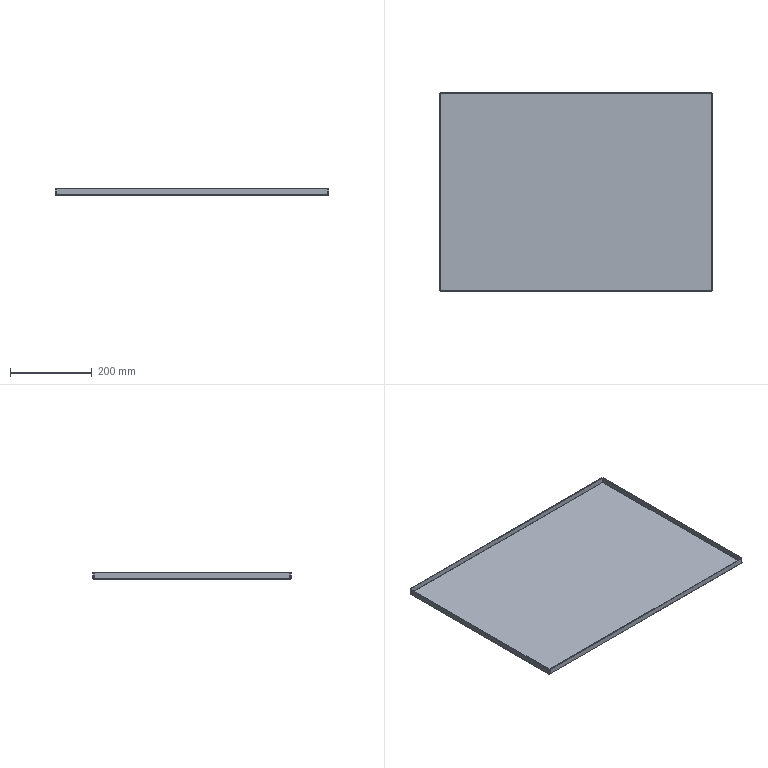Part | SolidWorks | 1 solid | 38 faces | box 670 x 485 x 15 mm | volume 707189 mm3 | plane 22 | spline 8 | cylinder 8 | commonest cylinder face diameters 0.2 x4 4.2 x4
STEP:
#1=CARTESIAN_POINT('',(332.9,-240.4,-2.));
#2=VERTEX_POINT('',#1);
#3=CARTESIAN_POINT('',(-332.9,-240.4,-2.));
#4=VERTEX_POINT('',#3);
#5=CARTESIAN_POINT('',(332.9,-240.4,-2.));
#6=DIRECTION('',(-1.,0.,0.));
#7=VECTOR('',#6,1000.);
#8=LINE('',#5,#7);
#9=EDGE_CURVE('',#2,#4,#8,.T.);
#10=ORIENTED_EDGE('',*,*,#9,.T.);
#11=CARTESIAN_POINT('',(-332.9,240.4,-2.));
#12=VERTEX_POINT('',#11);
#13=CARTESIAN_POINT('',(-332.9,-240.4,-2.));
#14=DIRECTION('',(0.,1.,0.));
#15=VECTOR('',#14,1000.);
#16=LINE('',#13,#15);
#17=EDGE_CURVE('',#4,#12,#16,.T.);
#18=ORIENTED_EDGE('',*,*,#17,.T.);
#19=CARTESIAN_POINT('',(332.9,240.4,-2.));
#20=VERTEX_POINT('',#19);
#21=CARTESIAN_POINT('',(-332.9,240.4,-2.));
#22=DIRECTION('',(1.,0.,0.));
#23=VECTOR('',#22,1000.);
#24=LINE('',#21,#23);
#25=EDGE_CURVE('',#12,#20,#24,.T.);
#26=ORIENTED_EDGE('',*,*,#25,.T.);
#27=CARTESIAN_POINT('',(332.9,240.4,-2.));
#28=DIRECTION('',(0.,-1.,0.));
#29=VECTOR('',#28,1000.);
#30=LINE('',#27,#29);
#31=EDGE_CURVE('',#20,#2,#30,.T.);
#32=ORIENTED_EDGE('',*,*,#31,.T.);
#33=EDGE_LOOP('',(#10,#18,#26,#32));
#34=FACE_OUTER_BOUND('',#33,.T.);
#35=CARTESIAN_POINT('',(0.,0.,-2.));
#36=DIRECTION('',(0.,0.,1.));
#37=DIRECTION('',(1.,0.,0.));
#38=AXIS2_PLACEMENT_3D('',#35,#36,#37);
#39=PLANE('',#38);
#40=ADVANCED_FACE('',(#34),#39,.F.);
#41=CARTESIAN_POINT('',(-332.9,-240.4,0.));
#42=VERTEX_POINT('',#41);
#43=CARTESIAN_POINT('',(-332.9,240.4,0.));
#44=VERTEX_POINT('',#43);
#45=CARTESIAN_POINT('',(-332.9,-240.4,0.));
#46=DIRECTION('',(0.,1.,0.));
#47=VECTOR('',#46,1000.);
#48=LINE('',#45,#47);
#49=EDGE_CURVE('',#42,#44,#48,.T.);
#50=ORIENTED_EDGE('',*,*,#49,.F.);
#51=CARTESIAN_POINT('',(332.9,-240.4,0.));
#52=VERTEX_POINT('',#51);
#53=CARTESIAN_POINT('',(332.9,-240.4,0.));
#54=DIRECTION('',(-1.,0.,0.));
#55=VECTOR('',#54,1000.);
#56=LINE('',#53,#55);
#57=EDGE_CURVE('',#52,#42,#56,.T.);
#58=ORIENTED_EDGE('',*,*,#57,.F.);
#59=CARTESIAN_POINT('',(332.9,240.4,0.));
#60=VERTEX_POINT('',#59);
#61=CARTESIAN_POINT('',(332.9,240.4,0.));
#62=DIRECTION('',(0.,-1.,0.));
#63=VECTOR('',#62,1000.);
#64=LINE('',#61,#63);
#65=EDGE_CURVE('',#60,#52,#64,.T.);
#66=ORIENTED_EDGE('',*,*,#65,.F.);
#67=CARTESIAN_POINT('',(-332.9,240.4,0.));
#68=DIRECTION('',(1.,0.,0.));
#69=VECTOR('',#68,1000.);
#70=LINE('',#67,#69);
#71=EDGE_CURVE('',#44,#60,#70,.T.);
#72=ORIENTED_EDGE('',*,*,#71,.F.);
#73=EDGE_LOOP('',(#50,#58,#66,#72));
#74=FACE_OUTER_BOUND('',#73,.T.);
#75=CARTESIAN_POINT('',(0.,0.,0.));
#76=DIRECTION('',(0.,0.,1.));
#77=DIRECTION('',(1.,0.,0.));
#78=AXIS2_PLACEMENT_3D('',#75,#76,#77);
#79=PLANE('',#78);
#80=ADVANCED_FACE('',(#74),#79,.T.);
#81=CARTESIAN_POINT('',(-335.,239.793,0.1));
#82=VERTEX_POINT('',#81);
#83=CARTESIAN_POINT('',(-333.,239.793,0.1));
#84=VERTEX_POINT('',#83);
#85=CARTESIAN_POINT('',(-333.,239.793,0.1));
#86=DIRECTION('',(1.,0.,0.));
#87=VECTOR('',#86,1000.);
#88=LINE('',#85,#87);
#89=EDGE_CURVE('',#82,#84,#88,.T.);
#90=ORIENTED_EDGE('',*,*,#89,.T.);
#91=CARTESIAN_POINT('',(-332.9,240.4,0.));
#92=CARTESIAN_POINT('',(-332.926,240.299,0.));
#93=CARTESIAN_POINT('',(-332.952,240.198,0.01078));
#94=CARTESIAN_POINT('',(-332.989,239.995,0.0478));
#95=CARTESIAN_POINT('',(-333.,239.894,0.07382));
#96=CARTESIAN_POINT('',(-333.,239.793,0.1));
#97=B_SPLINE_CURVE_WITH_KNOTS('',3,(#91,#92,#93,#94,#95,#96),.UNSPECIFIED.,.F.,.F.,(4,2,4),(0.,0.5,1.),.UNSPECIFIED.);
#98=EDGE_CURVE('',#44,#84,#97,.T.);
#99=ORIENTED_EDGE('',*,*,#98,.F.);
#100=CARTESIAN_POINT('',(-332.9,240.4,0.));
#101=DIRECTION('',(0.,0.,-1.));
#102=VECTOR('',#101,1000.);
#103=LINE('',#100,#102);
#104=EDGE_CURVE('',#44,#12,#103,.T.);
#105=ORIENTED_EDGE('',*,*,#104,.T.);
#106=CARTESIAN_POINT('',(-332.9,240.4,-2.));
#107=CARTESIAN_POINT('',(-333.039,240.374,-2.));
#108=CARTESIAN_POINT('',(-333.175,240.349,-1.986));
#109=CARTESIAN_POINT('',(-333.443,240.299,-1.933));
#110=CARTESIAN_POINT('',(-333.576,240.274,-1.893));
#111=CARTESIAN_POINT('',(-333.831,240.223,-1.787));
#112=CARTESIAN_POINT('',(-333.951,240.198,-1.723));
#113=CARTESIAN_POINT('',(-334.179,240.147,-1.571));
#114=CARTESIAN_POINT('',(-334.287,240.122,-1.482));
#115=CARTESIAN_POINT('',(-334.481,240.071,-1.289));
#116=CARTESIAN_POINT('',(-334.568,240.046,-1.183));
#117=CARTESIAN_POINT('',(-334.721,239.996,-0.9542));
#118=CARTESIAN_POINT('',(-334.787,239.97,-0.8315));
#119=CARTESIAN_POINT('',(-334.944,239.895,-0.4527));
#120=CARTESIAN_POINT('',(-335.,239.844,-0.1773));
#121=CARTESIAN_POINT('',(-335.,239.793,0.1));
#122=B_SPLINE_CURVE_WITH_KNOTS('',3,(#106,#107,#108,#109,#110,#111,#112,#113,#114,#115,#116,#117,#118,#119,#120,#121),.UNSPECIFIED.,.F.,.F.,(4,2,2,2,2,2,2,4),(0.,0.0004169,0.0008339,0.001251,0.001668,0.002085,0.002502,0.003336),.UNSPECIFIED.);
#123=EDGE_CURVE('',#12,#82,#122,.T.);
#124=ORIENTED_EDGE('',*,*,#123,.T.);
#125=EDGE_LOOP('',(#90,#99,#105,#124));
#126=FACE_OUTER_BOUND('',#125,.T.);
#127=CARTESIAN_POINT('',(-332.9,240.4,-2.02));
#128=CARTESIAN_POINT('',(-333.178,240.349,-2.02));
#129=CARTESIAN_POINT('',(-333.455,240.299,-1.965));
#130=CARTESIAN_POINT('',(-333.968,240.198,-1.752));
#131=CARTESIAN_POINT('',(-334.203,240.147,-1.595));
#132=CARTESIAN_POINT('',(-334.595,240.046,-1.203));
#133=CARTESIAN_POINT('',(-334.752,239.995,-0.9677));
#134=CARTESIAN_POINT('',(-334.965,239.894,-0.4549));
#135=CARTESIAN_POINT('',(-335.02,239.843,-0.1776));
#136=CARTESIAN_POINT('',(-335.02,239.793,0.1));
#137=CARTESIAN_POINT('',(-332.9,240.4,-2.));
#138=CARTESIAN_POINT('',(-333.175,240.349,-2.));
#139=CARTESIAN_POINT('',(-333.45,240.299,-1.945));
#140=CARTESIAN_POINT('',(-333.958,240.198,-1.735));
#141=CARTESIAN_POINT('',(-334.191,240.147,-1.579));
#142=CARTESIAN_POINT('',(-334.579,240.046,-1.191));
#143=CARTESIAN_POINT('',(-334.735,239.995,-0.9576));
#144=CARTESIAN_POINT('',(-334.945,239.894,-0.4497));
#145=CARTESIAN_POINT('',(-335.,239.843,-0.1749));
#146=CARTESIAN_POINT('',(-335.,239.793,0.1));
#147=CARTESIAN_POINT('',(-332.9,240.4,0.));
#148=CARTESIAN_POINT('',(-332.913,240.349,0.));
#149=CARTESIAN_POINT('',(-332.926,240.299,0.002603));
#150=CARTESIAN_POINT('',(-332.95,240.198,0.01262));
#151=CARTESIAN_POINT('',(-332.961,240.147,0.02003));
#152=CARTESIAN_POINT('',(-332.98,240.046,0.03855));
#153=CARTESIAN_POINT('',(-332.987,239.995,0.04964));
#154=CARTESIAN_POINT('',(-332.997,239.894,0.07383));
#155=CARTESIAN_POINT('',(-333.,239.843,0.08691));
#156=CARTESIAN_POINT('',(-333.,239.793,0.1));
#157=B_SPLINE_SURFACE_WITH_KNOTS('',1,3,((#127,#128,#129,#130,#131,#132,#133,#134,#135,#136),(#137,#138,#139,#140,#141,#142,#143,#144,#145,#146),(#147,#148,#149,#150,#151,#152,#153,#154,#155,#156)),.UNSPECIFIED.,.F.,.F.,.F.,(2,1,2),(4,2,2,2,4),(-0.01,0.,1.),(0.,0.25,0.5,0.75,1.),.UNSPECIFIED.);
#158=ADVANCED_FACE('',(#126),#157,.F.);
#159=CARTESIAN_POINT('',(-333.,-239.793,0.1));
#160=VERTEX_POINT('',#159);
#161=CARTESIAN_POINT('',(-333.,-239.793,0.1));
#162=CARTESIAN_POINT('',(-333.,-239.894,0.07382));
#163=CARTESIAN_POINT('',(-332.989,-239.995,0.0478));
#164=CARTESIAN_POINT('',(-332.952,-240.198,0.01078));
#165=CARTESIAN_POINT('',(-332.926,-240.299,0.));
#166=CARTESIAN_POINT('',(-332.9,-240.4,0.));
#167=B_SPLINE_CURVE_WITH_KNOTS('',3,(#161,#162,#163,#164,#165,#166),.UNSPECIFIED.,.F.,.F.,(4,2,4),(0.,0.5,1.),.UNSPECIFIED.);
#168=EDGE_CURVE('',#160,#42,#167,.T.);
#169=ORIENTED_EDGE('',*,*,#168,.F.);
#170=CARTESIAN_POINT('',(-335.,-239.793,0.1));
#171=VERTEX_POINT('',#170);
#172=CARTESIAN_POINT('',(-333.,-239.793,0.1));
#173=DIRECTION('',(1.,0.,0.));
#174=VECTOR('',#173,1000.);
#175=LINE('',#172,#174);
#176=EDGE_CURVE('',#171,#160,#175,.T.);
#177=ORIENTED_EDGE('',*,*,#176,.F.);
#178=CARTESIAN_POINT('',(-335.,-239.793,0.1));
#179=CARTESIAN_POINT('',(-335.,-239.818,-0.03865));
#180=CARTESIAN_POINT('',(-334.986,-239.844,-0.175));
#181=CARTESIAN_POINT('',(-334.933,-239.894,-0.4432));
#182=CARTESIAN_POINT('',(-334.893,-239.919,-0.5764));
#183=CARTESIAN_POINT('',(-334.787,-239.97,-0.8308));
#184=CARTESIAN_POINT('',(-334.723,-239.995,-0.9514));
#185=CARTESIAN_POINT('',(-334.571,-240.045,-1.179));
#186=CARTESIAN_POINT('',(-334.482,-240.071,-1.287));
#187=CARTESIAN_POINT('',(-334.289,-240.122,-1.481));
#188=CARTESIAN_POINT('',(-334.183,-240.147,-1.568));
#189=CARTESIAN_POINT('',(-333.954,-240.197,-1.721));
#190=CARTESIAN_POINT('',(-333.832,-240.223,-1.787));
#191=CARTESIAN_POINT('',(-333.453,-240.298,-1.944));
#192=CARTESIAN_POINT('',(-333.177,-240.349,-2.));
#193=CARTESIAN_POINT('',(-332.9,-240.4,-2.));
#194=B_SPLINE_CURVE_WITH_KNOTS('',3,(#178,#179,#180,#181,#182,#183,#184,#185,#186,#187,#188,#189,#190,#191,#192,#193),.UNSPECIFIED.,.F.,.F.,(4,2,2,2,2,2,2,4),(0.,0.0004169,0.0008339,0.001251,0.001668,0.002085,0.002502,0.003336),.UNSPECIFIED.);
#195=EDGE_CURVE('',#171,#4,#194,.T.);
#196=ORIENTED_EDGE('',*,*,#195,.T.);
#197=CARTESIAN_POINT('',(-332.9,-240.4,0.));
#198=DIRECTION('',(0.,0.,-1.));
#199=VECTOR('',#198,1000.);
#200=LINE('',#197,#199);
#201=EDGE_CURVE('',#42,#4,#200,.T.);
#202=ORIENTED_EDGE('',*,*,#201,.F.);
#203=EDGE_LOOP('',(#169,#177,#196,#202));
#204=FACE_OUTER_BOUND('',#203,.T.);
#205=CARTESIAN_POINT('',(-335.02,-239.793,0.1));
#206=CARTESIAN_POINT('',(-335.02,-239.843,-0.1776));
#207=CARTESIAN_POINT('',(-334.965,-239.894,-0.4549));
#208=CARTESIAN_POINT('',(-334.752,-239.995,-0.9677));
#209=CARTESIAN_POINT('',(-334.595,-240.046,-1.203));
#210=CARTESIAN_POINT('',(-334.203,-240.147,-1.595));
#211=CARTESIAN_POINT('',(-333.968,-240.198,-1.752));
#212=CARTESIAN_POINT('',(-333.455,-240.299,-1.965));
#213=CARTESIAN_POINT('',(-333.178,-240.349,-2.02));
#214=CARTESIAN_POINT('',(-332.9,-240.4,-2.02));
#215=CARTESIAN_POINT('',(-335.,-239.793,0.1));
#216=CARTESIAN_POINT('',(-335.,-239.843,-0.1749));
#217=CARTESIAN_POINT('',(-334.945,-239.894,-0.4497));
#218=CARTESIAN_POINT('',(-334.735,-239.995,-0.9576));
#219=CARTESIAN_POINT('',(-334.579,-240.046,-1.191));
#220=CARTESIAN_POINT('',(-334.191,-240.147,-1.579));
#221=CARTESIAN_POINT('',(-333.958,-240.198,-1.735));
#222=CARTESIAN_POINT('',(-333.45,-240.299,-1.945));
#223=CARTESIAN_POINT('',(-333.175,-240.349,-2.));
#224=CARTESIAN_POINT('',(-332.9,-240.4,-2.));
#225=CARTESIAN_POINT('',(-333.,-239.793,0.1));
#226=CARTESIAN_POINT('',(-333.,-239.843,0.08691));
#227=CARTESIAN_POINT('',(-332.997,-239.894,0.07383));
#228=CARTESIAN_POINT('',(-332.987,-239.995,0.04964));
#229=CARTESIAN_POINT('',(-332.98,-240.046,0.03855));
#230=CARTESIAN_POINT('',(-332.961,-240.147,0.02003));
#231=CARTESIAN_POINT('',(-332.95,-240.198,0.01262));
#232=CARTESIAN_POINT('',(-332.926,-240.299,0.002603));
#233=CARTESIAN_POINT('',(-332.913,-240.349,0.));
#234=CARTESIAN_POINT('',(-332.9,-240.4,0.));
#235=B_SPLINE_SURFACE_WITH_KNOTS('',1,3,((#205,#206,#207,#208,#209,#210,#211,#212,#213,#214),(#215,#216,#217,#218,#219,#220,#221,#222,#223,#224),(#225,#226,#227,#228,#229,#230,#231,#232,#233,#234)),.UNSPECIFIED.,.F.,.F.,.F.,(2,1,2),(4,2,2,2,4),(-0.01,0.,1.),(0.,0.25,0.5,0.75,1.),.UNSPECIFIED.);
#236=ADVANCED_FACE('',(#204),#235,.F.);
#237=ORIENTED_EDGE('',*,*,#17,.F.);
#238=ORIENTED_EDGE('',*,*,#195,.F.);
#239=CARTESIAN_POINT('',(-335.,242.5,0.1));
#240=DIRECTION('',(0.,1.,0.));
#241=VECTOR('',#240,1000.);
#242=LINE('',#239,#241);
#243=EDGE_CURVE('',#171,#82,#242,.T.);
#244=ORIENTED_EDGE('',*,*,#243,.T.);
#245=ORIENTED_EDGE('',*,*,#123,.F.);
#246=EDGE_LOOP('',(#237,#238,#244,#245));
#247=FACE_OUTER_BOUND('',#246,.T.);
#248=CARTESIAN_POINT('',(-332.9,-240.4,0.1));
#249=DIRECTION('',(0.,-1.,0.));
#250=DIRECTION('',(-1.,0.,0.));
#251=AXIS2_PLACEMENT_3D('',#248,#249,#250);
#252=CYLINDRICAL_SURFACE('',#251,2.1);
#253=ADVANCED_FACE('',(#247),#252,.T.);
#254=ORIENTED_EDGE('',*,*,#49,.T.);
#255=ORIENTED_EDGE('',*,*,#98,.T.);
#256=CARTESIAN_POINT('',(-333.,242.5,0.1));
#257=DIRECTION('',(0.,-1.,0.));
#258=VECTOR('',#257,1000.);
#259=LINE('',#256,#258);
#260=EDGE_CURVE('',#84,#160,#259,.T.);
#261=ORIENTED_EDGE('',*,*,#260,.T.);
#262=ORIENTED_EDGE('',*,*,#168,.T.);
#263=EDGE_LOOP('',(#254,#255,#261,#262));
#264=FACE_OUTER_BOUND('',#263,.T.);
#265=CARTESIAN_POINT('',(-332.9,-240.4,0.1));
#266=DIRECTION('',(0.,-1.,0.));
#267=DIRECTION('',(-1.,0.,0.));
#268=AXIS2_PLACEMENT_3D('',#265,#266,#267);
#269=CYLINDRICAL_SURFACE('',#268,0.1);
#270=ADVANCED_FACE('',(#264),#269,.F.);
#271=CARTESIAN_POINT('',(-335.,239.793,13.));
#272=VERTEX_POINT('',#271);
#273=CARTESIAN_POINT('',(-335.,239.793,0.));
#274=DIRECTION('',(0.,0.,1.));
#275=VECTOR('',#274,1000.);
#276=LINE('',#273,#275);
#277=EDGE_CURVE('',#82,#272,#276,.T.);
#278=ORIENTED_EDGE('',*,*,#277,.T.);
#279=CARTESIAN_POINT('',(-333.,239.793,13.));
#280=VERTEX_POINT('',#279);
#281=CARTESIAN_POINT('',(-333.,239.793,13.));
#282=DIRECTION('',(1.,0.,0.));
#283=VECTOR('',#282,1000.);
#284=LINE('',#281,#283);
#285=EDGE_CURVE('',#272,#280,#284,.T.);
#286=ORIENTED_EDGE('',*,*,#285,.T.);
#287=CARTESIAN_POINT('',(-333.,239.793,0.));
#288=DIRECTION('',(0.,0.,1.));
#289=VECTOR('',#288,1000.);
#290=LINE('',#287,#289);
#291=EDGE_CURVE('',#84,#280,#290,.T.);
#292=ORIENTED_EDGE('',*,*,#291,.F.);
#293=ORIENTED_EDGE('',*,*,#89,.F.);
#294=EDGE_LOOP('',(#278,#286,#292,#293));
#295=FACE_OUTER_BOUND('',#294,.T.);
#296=CARTESIAN_POINT('',(-333.,239.793,0.));
#297=DIRECTION('',(0.,1.,0.));
#298=DIRECTION('',(0.,0.,1.));
#299=AXIS2_PLACEMENT_3D('',#296,#297,#298);
#300=PLANE('',#299);
#301=ADVANCED_FACE('',(#295),#300,.T.);
#302=ORIENTED_EDGE('',*,*,#243,.F.);
#303=CARTESIAN_POINT('',(-335.,-239.793,13.));
#304=VERTEX_POINT('',#303);
#305=CARTESIAN_POINT('',(-335.,-239.793,0.));
#306=DIRECTION('',(0.,0.,1.));
#307=VECTOR('',#306,1000.);
#308=LINE('',#305,#307);
#309=EDGE_CURVE('',#171,#304,#308,.T.);
#310=ORIENTED_EDGE('',*,*,#309,.T.);
#311=CARTESIAN_POINT('',(-335.,0.,13.));
#312=DIRECTION('',(0.,1.,0.));
#313=VECTOR('',#312,1000.);
#314=LINE('',#311,#313);
#315=EDGE_CURVE('',#304,#272,#314,.T.);
#316=ORIENTED_EDGE('',*,*,#315,.T.);
#317=ORIENTED_EDGE('',*,*,#277,.F.);
#318=EDGE_LOOP('',(#302,#310,#316,#317));
#319=FACE_OUTER_BOUND('',#318,.T.);
#320=CARTESIAN_POINT('',(-335.,0.,0.));
#321=DIRECTION('',(1.,0.,0.));
#322=DIRECTION('',(0.,0.,-1.));
#323=AXIS2_PLACEMENT_3D('',#320,#321,#322);
#324=PLANE('',#323);
#325=ADVANCED_FACE('',(#319),#324,.F.);
#326=CARTESIAN_POINT('',(-333.,-239.793,13.));
#327=VERTEX_POINT('',#326);
#328=CARTESIAN_POINT('',(-333.,-239.793,0.));
#329=DIRECTION('',(0.,0.,1.));
#330=VECTOR('',#329,1000.);
#331=LINE('',#328,#330);
#332=EDGE_CURVE('',#160,#327,#331,.T.);
#333=ORIENTED_EDGE('',*,*,#332,.F.);
#334=ORIENTED_EDGE('',*,*,#260,.F.);
#335=ORIENTED_EDGE('',*,*,#291,.T.);
#336=CARTESIAN_POINT('',(-333.,242.5,13.));
#337=DIRECTION('',(0.,1.,0.));
#338=VECTOR('',#337,1000.);
#339=LINE('',#336,#338);
#340=EDGE_CURVE('',#327,#280,#339,.T.);
#341=ORIENTED_EDGE('',*,*,#340,.F.);
#342=EDGE_LOOP('',(#333,#334,#335,#341));
#343=FACE_OUTER_BOUND('',#342,.T.);
#344=CARTESIAN_POINT('',(-333.,0.,0.));
#345=DIRECTION('',(1.,0.,0.));
#346=DIRECTION('',(0.,0.,-1.));
#347=AXIS2_PLACEMENT_3D('',#344,#345,#346);
#348=PLANE('',#347);
#349=ADVANCED_FACE('',(#343),#348,.T.);
#350=ORIENTED_EDGE('',*,*,#315,.F.);
#351=CARTESIAN_POINT('',(-335.,-239.793,13.));
#352=DIRECTION('',(1.,0.,0.));
#353=VECTOR('',#352,1000.);
#354=LINE('',#351,#353);
#355=EDGE_CURVE('',#304,#327,#354,.T.);
#356=ORIENTED_EDGE('',*,*,#355,.T.);
#357=ORIENTED_EDGE('',*,*,#340,.T.);
#358=ORIENTED_EDGE('',*,*,#285,.F.);
#359=EDGE_LOOP('',(#350,#356,#357,#358));
#360=FACE_OUTER_BOUND('',#359,.T.);
#361=CARTESIAN_POINT('',(-335.,242.5,13.));
#362=DIRECTION('',(0.,0.,-1.));
#363=DIRECTION('',(-1.,0.,0.));
#364=AXIS2_PLACEMENT_3D('',#361,#362,#363);
#365=PLANE('',#364);
#366=ADVANCED_FACE('',(#360),#365,.F.);
#367=ORIENTED_EDGE('',*,*,#355,.F.);
#368=ORIENTED_EDGE('',*,*,#309,.F.);
#369=ORIENTED_EDGE('',*,*,#176,.T.);
#370=ORIENTED_EDGE('',*,*,#332,.T.);
#371=EDGE_LOOP('',(#367,#368,#369,#370));
#372=FACE_OUTER_BOUND('',#371,.T.);
#373=CARTESIAN_POINT('',(-333.,-239.793,0.));
#374=DIRECTION('',(0.,1.,0.));
#375=DIRECTION('',(0.,0.,1.));
#376=AXIS2_PLACEMENT_3D('',#373,#374,#375);
#377=PLANE('',#376);
#378=ADVANCED_FACE('',(#372),#377,.F.);
#379=CARTESIAN_POINT('',(332.293,242.5,0.1));
#380=VERTEX_POINT('',#379);
#381=CARTESIAN_POINT('',(332.293,240.5,0.1));
#382=VERTEX_POINT('',#381);
#383=CARTESIAN_POINT('',(332.293,240.5,0.1));
#384=DIRECTION('',(0.,-1.,0.));
#385=VECTOR('',#384,1000.);
#386=LINE('',#383,#385);
#387=EDGE_CURVE('',#380,#382,#386,.T.);
#388=ORIENTED_EDGE('',*,*,#387,.T.);
#389=CARTESIAN_POINT('',(332.9,240.4,0.));
#390=CARTESIAN_POINT('',(332.799,240.426,0.));
#391=CARTESIAN_POINT('',(332.698,240.452,0.01078));
#392=CARTESIAN_POINT('',(332.495,240.489,0.0478));
#393=CARTESIAN_POINT('',(332.394,240.5,0.07382));
#394=CARTESIAN_POINT('',(332.293,240.5,0.1));
#395=B_SPLINE_CURVE_WITH_KNOTS('',3,(#389,#390,#391,#392,#393,#394),.UNSPECIFIED.,.F.,.F.,(4,2,4),(0.,0.5,1.),.UNSPECIFIED.);
#396=EDGE_CURVE('',#60,#382,#395,.T.);
#397=ORIENTED_EDGE('',*,*,#396,.F.);
#398=CARTESIAN_POINT('',(332.9,240.4,0.));
#399=DIRECTION('',(0.,0.,-1.));
#400=VECTOR('',#399,1000.);
#401=LINE('',#398,#400);
#402=EDGE_CURVE('',#60,#20,#401,.T.);
#403=ORIENTED_EDGE('',*,*,#402,.T.);
#404=CARTESIAN_POINT('',(332.9,240.4,-2.));
#405=CARTESIAN_POINT('',(332.874,240.539,-2.));
#406=CARTESIAN_POINT('',(332.849,240.675,-1.986));
#407=CARTESIAN_POINT('',(332.799,240.943,-1.933));
#408=CARTESIAN_POINT('',(332.774,241.076,-1.893));
#409=CARTESIAN_POINT('',(332.723,241.331,-1.787));
#410=CARTESIAN_POINT('',(332.698,241.451,-1.723));
#411=CARTESIAN_POINT('',(332.647,241.679,-1.571));
#412=CARTESIAN_POINT('',(332.622,241.787,-1.482));
#413=CARTESIAN_POINT('',(332.571,241.981,-1.289));
#414=CARTESIAN_POINT('',(332.546,242.068,-1.183));
#415=CARTESIAN_POINT('',(332.496,242.221,-0.9542));
#416=CARTESIAN_POINT('',(332.47,242.287,-0.8315));
#417=CARTESIAN_POINT('',(332.395,242.444,-0.4527));
#418=CARTESIAN_POINT('',(332.344,242.5,-0.1773));
#419=CARTESIAN_POINT('',(332.293,242.5,0.1));
#420=B_SPLINE_CURVE_WITH_KNOTS('',3,(#404,#405,#406,#407,#408,#409,#410,#411,#412,#413,#414,#415,#416,#417,#418,#419),.UNSPECIFIED.,.F.,.F.,(4,2,2,2,2,2,2,4),(0.,0.0004169,0.0008339,0.001251,0.001668,0.002085,0.002502,0.003336),.UNSPECIFIED.);
#421=EDGE_CURVE('',#20,#380,#420,.T.);
#422=ORIENTED_EDGE('',*,*,#421,.T.);
#423=EDGE_LOOP('',(#388,#397,#403,#422));
#424=FACE_OUTER_BOUND('',#423,.T.);
#425=CARTESIAN_POINT('',(332.9,240.4,-2.02));
#426=CARTESIAN_POINT('',(332.849,240.678,-2.02));
#427=CARTESIAN_POINT('',(332.799,240.955,-1.965));
#428=CARTESIAN_POINT('',(332.698,241.468,-1.752));
#429=CARTESIAN_POINT('',(332.647,241.703,-1.595));
#430=CARTESIAN_POINT('',(332.546,242.095,-1.203));
#431=CARTESIAN_POINT('',(332.495,242.252,-0.9677));
#432=CARTESIAN_POINT('',(332.394,242.465,-0.4549));
#433=CARTESIAN_POINT('',(332.343,242.52,-0.1776));
#434=CARTESIAN_POINT('',(332.293,242.52,0.1));
#435=CARTESIAN_POINT('',(332.9,240.4,-2.));
#436=CARTESIAN_POINT('',(332.849,240.675,-2.));
#437=CARTESIAN_POINT('',(332.799,240.95,-1.945));
#438=CARTESIAN_POINT('',(332.698,241.458,-1.735));
#439=CARTESIAN_POINT('',(332.647,241.691,-1.579));
#440=CARTESIAN_POINT('',(332.546,242.079,-1.191));
#441=CARTESIAN_POINT('',(332.495,242.235,-0.9576));
#442=CARTESIAN_POINT('',(332.394,242.445,-0.4497));
#443=CARTESIAN_POINT('',(332.343,242.5,-0.1749));
#444=CARTESIAN_POINT('',(332.293,242.5,0.1));
#445=CARTESIAN_POINT('',(332.9,240.4,0.));
#446=CARTESIAN_POINT('',(332.849,240.413,0.));
#447=CARTESIAN_POINT('',(332.799,240.426,0.002603));
#448=CARTESIAN_POINT('',(332.698,240.45,0.01262));
#449=CARTESIAN_POINT('',(332.647,240.461,0.02003));
#450=CARTESIAN_POINT('',(332.546,240.48,0.03855));
#451=CARTESIAN_POINT('',(332.495,240.487,0.04964));
#452=CARTESIAN_POINT('',(332.394,240.497,0.07383));
#453=CARTESIAN_POINT('',(332.343,240.5,0.08691));
#454=CARTESIAN_POINT('',(332.293,240.5,0.1));
#455=B_SPLINE_SURFACE_WITH_KNOTS('',1,3,((#425,#426,#427,#428,#429,#430,#431,#432,#433,#434),(#435,#436,#437,#438,#439,#440,#441,#442,#443,#444),(#445,#446,#447,#448,#449,#450,#451,#452,#453,#454)),.UNSPECIFIED.,.F.,.F.,.F.,(2,1,2),(4,2,2,2,4),(-0.01,0.,1.),(0.,0.25,0.5,0.75,1.),.UNSPECIFIED.);
#456=ADVANCED_FACE('',(#424),#455,.F.);
#457=CARTESIAN_POINT('',(-332.293,240.5,0.1));
#458=VERTEX_POINT('',#457);
#459=CARTESIAN_POINT('',(-332.293,240.5,0.1));
#460=CARTESIAN_POINT('',(-332.394,240.5,0.07382));
#461=CARTESIAN_POINT('',(-332.495,240.489,0.0478));
#462=CARTESIAN_POINT('',(-332.698,240.452,0.01078));
#463=CARTESIAN_POINT('',(-332.799,240.426,0.));
#464=CARTESIAN_POINT('',(-332.9,240.4,0.));
#465=B_SPLINE_CURVE_WITH_KNOTS('',3,(#459,#460,#461,#462,#463,#464),.UNSPECIFIED.,.F.,.F.,(4,2,4),(0.,0.5,1.),.UNSPECIFIED.);
#466=EDGE_CURVE('',#458,#44,#465,.T.);
#467=ORIENTED_EDGE('',*,*,#466,.F.);
#468=CARTESIAN_POINT('',(-332.293,242.5,0.1));
#469=VERTEX_POINT('',#468);
#470=CARTESIAN_POINT('',(-332.293,240.5,0.1));
#471=DIRECTION('',(0.,-1.,0.));
#472=VECTOR('',#471,1000.);
#473=LINE('',#470,#472);
#474=EDGE_CURVE('',#469,#458,#473,.T.);
#475=ORIENTED_EDGE('',*,*,#474,.F.);
#476=CARTESIAN_POINT('',(-332.293,242.5,0.1));
#477=CARTESIAN_POINT('',(-332.318,242.5,-0.03865));
#478=CARTESIAN_POINT('',(-332.344,242.486,-0.175));
#479=CARTESIAN_POINT('',(-332.394,242.433,-0.4432));
#480=CARTESIAN_POINT('',(-332.419,242.393,-0.5764));
#481=CARTESIAN_POINT('',(-332.47,242.287,-0.8308));
#482=CARTESIAN_POINT('',(-332.495,242.223,-0.9514));
#483=CARTESIAN_POINT('',(-332.545,242.071,-1.179));
#484=CARTESIAN_POINT('',(-332.571,241.982,-1.287));
#485=CARTESIAN_POINT('',(-332.622,241.789,-1.481));
#486=CARTESIAN_POINT('',(-332.647,241.683,-1.568));
#487=CARTESIAN_POINT('',(-332.697,241.454,-1.721));
#488=CARTESIAN_POINT('',(-332.723,241.332,-1.787));
#489=CARTESIAN_POINT('',(-332.798,240.953,-1.944));
#490=CARTESIAN_POINT('',(-332.849,240.677,-2.));
#491=CARTESIAN_POINT('',(-332.9,240.4,-2.));
#492=B_SPLINE_CURVE_WITH_KNOTS('',3,(#476,#477,#478,#479,#480,#481,#482,#483,#484,#485,#486,#487,#488,#489,#490,#491),.UNSPECIFIED.,.F.,.F.,(4,2,2,2,2,2,2,4),(0.,0.0004169,0.0008339,0.001251,0.001668,0.002085,0.002502,0.003336),.UNSPECIFIED.);
#493=EDGE_CURVE('',#469,#12,#492,.T.);
#494=ORIENTED_EDGE('',*,*,#493,.T.);
#495=ORIENTED_EDGE('',*,*,#104,.F.);
#496=EDGE_LOOP('',(#467,#475,#494,#495));
#497=FACE_OUTER_BOUND('',#496,.T.);
#498=CARTESIAN_POINT('',(-332.293,242.52,0.1));
#499=CARTESIAN_POINT('',(-332.343,242.52,-0.1776));
#500=CARTESIAN_POINT('',(-332.394,242.465,-0.4549));
#501=CARTESIAN_POINT('',(-332.495,242.252,-0.9677));
#502=CARTESIAN_POINT('',(-332.546,242.095,-1.203));
#503=CARTESIAN_POINT('',(-332.647,241.703,-1.595));
#504=CARTESIAN_POINT('',(-332.698,241.468,-1.752));
#505=CARTESIAN_POINT('',(-332.799,240.955,-1.965));
#506=CARTESIAN_POINT('',(-332.849,240.678,-2.02));
#507=CARTESIAN_POINT('',(-332.9,240.4,-2.02));
#508=CARTESIAN_POINT('',(-332.293,242.5,0.1));
#509=CARTESIAN_POINT('',(-332.343,242.5,-0.1749));
#510=CARTESIAN_POINT('',(-332.394,242.445,-0.4497));
#511=CARTESIAN_POINT('',(-332.495,242.235,-0.9576));
#512=CARTESIAN_POINT('',(-332.546,242.079,-1.191));
#513=CARTESIAN_POINT('',(-332.647,241.691,-1.579));
#514=CARTESIAN_POINT('',(-332.698,241.458,-1.735));
#515=CARTESIAN_POINT('',(-332.799,240.95,-1.945));
#516=CARTESIAN_POINT('',(-332.849,240.675,-2.));
#517=CARTESIAN_POINT('',(-332.9,240.4,-2.));
#518=CARTESIAN_POINT('',(-332.293,240.5,0.1));
#519=CARTESIAN_POINT('',(-332.343,240.5,0.08691));
#520=CARTESIAN_POINT('',(-332.394,240.497,0.07383));
#521=CARTESIAN_POINT('',(-332.495,240.487,0.04964));
#522=CARTESIAN_POINT('',(-332.546,240.48,0.03855));
#523=CARTESIAN_POINT('',(-332.647,240.461,0.02003));
#524=CARTESIAN_POINT('',(-332.698,240.45,0.01262));
#525=CARTESIAN_POINT('',(-332.799,240.426,0.002603));
#526=CARTESIAN_POINT('',(-332.849,240.413,0.));
#527=CARTESIAN_POINT('',(-332.9,240.4,0.));
#528=B_SPLINE_SURFACE_WITH_KNOTS('',1,3,((#498,#499,#500,#501,#502,#503,#504,#505,#506,#507),(#508,#509,#510,#511,#512,#513,#514,#515,#516,#517),(#518,#519,#520,#521,#522,#523,#524,#525,#526,#527)),.UNSPECIFIED.,.F.,.F.,.F.,(2,1,2),(4,2,2,2,4),(-0.01,0.,1.),(0.,0.25,0.5,0.75,1.),.UNSPECIFIED.);
#529=ADVANCED_FACE('',(#497),#528,.F.);
#530=ORIENTED_EDGE('',*,*,#25,.F.);
#531=ORIENTED_EDGE('',*,*,#493,.F.);
#532=CARTESIAN_POINT('',(335.,242.5,0.1));
#533=DIRECTION('',(1.,0.,0.));
#534=VECTOR('',#533,1000.);
#535=LINE('',#532,#534);
#536=EDGE_CURVE('',#469,#380,#535,.T.);
#537=ORIENTED_EDGE('',*,*,#536,.T.);
#538=ORIENTED_EDGE('',*,*,#421,.F.);
#539=EDGE_LOOP('',(#530,#531,#537,#538));
#540=FACE_OUTER_BOUND('',#539,.T.);
#541=CARTESIAN_POINT('',(-332.9,240.4,0.1));
#542=DIRECTION('',(-1.,0.,0.));
#543=DIRECTION('',(0.,1.,0.));
#544=AXIS2_PLACEMENT_3D('',#541,#542,#543);
#545=CYLINDRICAL_SURFACE('',#544,2.1);
#546=ADVANCED_FACE('',(#540),#545,.T.);
#547=ORIENTED_EDGE('',*,*,#71,.T.);
#548=ORIENTED_EDGE('',*,*,#396,.T.);
#549=CARTESIAN_POINT('',(335.,240.5,0.1));
#550=DIRECTION('',(-1.,0.,0.));
#551=VECTOR('',#550,1000.);
#552=LINE('',#549,#551);
#553=EDGE_CURVE('',#382,#458,#552,.T.);
#554=ORIENTED_EDGE('',*,*,#553,.T.);
#555=ORIENTED_EDGE('',*,*,#466,.T.);
#556=EDGE_LOOP('',(#547,#548,#554,#555));
#557=FACE_OUTER_BOUND('',#556,.T.);
#558=CARTESIAN_POINT('',(-332.9,240.4,0.1));
#559=DIRECTION('',(-1.,0.,0.));
#560=DIRECTION('',(0.,1.,0.));
#561=AXIS2_PLACEMENT_3D('',#558,#559,#560);
#562=CYLINDRICAL_SURFACE('',#561,0.1);
#563=ADVANCED_FACE('',(#557),#562,.F.);
#564=CARTESIAN_POINT('',(332.293,242.5,13.));
#565=VERTEX_POINT('',#564);
#566=CARTESIAN_POINT('',(332.293,242.5,0.));
#567=DIRECTION('',(0.,0.,1.));
#568=VECTOR('',#567,1000.);
#569=LINE('',#566,#568);
#570=EDGE_CURVE('',#380,#565,#569,.T.);
#571=ORIENTED_EDGE('',*,*,#570,.T.);
#572=CARTESIAN_POINT('',(332.293,240.5,13.));
#573=VERTEX_POINT('',#572);
#574=CARTESIAN_POINT('',(332.293,240.5,13.));
#575=DIRECTION('',(0.,-1.,0.));
#576=VECTOR('',#575,1000.);
#577=LINE('',#574,#576);
#578=EDGE_CURVE('',#565,#573,#577,.T.);
#579=ORIENTED_EDGE('',*,*,#578,.T.);
#580=CARTESIAN_POINT('',(332.293,240.5,0.));
#581=DIRECTION('',(0.,0.,1.));
#582=VECTOR('',#581,1000.);
#583=LINE('',#580,#582);
#584=EDGE_CURVE('',#382,#573,#583,.T.);
#585=ORIENTED_EDGE('',*,*,#584,.F.);
#586=ORIENTED_EDGE('',*,*,#387,.F.);
#587=EDGE_LOOP('',(#571,#579,#585,#586));
#588=FACE_OUTER_BOUND('',#587,.T.);
#589=CARTESIAN_POINT('',(332.293,240.5,0.));
#590=DIRECTION('',(1.,0.,0.));
#591=DIRECTION('',(0.,0.,-1.));
#592=AXIS2_PLACEMENT_3D('',#589,#590,#591);
#593=PLANE('',#592);
#594=ADVANCED_FACE('',(#588),#593,.T.);
#595=ORIENTED_EDGE('',*,*,#536,.F.);
#596=CARTESIAN_POINT('',(-332.293,242.5,13.));
#597=VERTEX_POINT('',#596);
#598=CARTESIAN_POINT('',(-332.293,242.5,0.));
#599=DIRECTION('',(0.,0.,1.));
#600=VECTOR('',#599,1000.);
#601=LINE('',#598,#600);
#602=EDGE_CURVE('',#469,#597,#601,.T.);
#603=ORIENTED_EDGE('',*,*,#602,.T.);
#604=CARTESIAN_POINT('',(0.,242.5,13.));
#605=DIRECTION('',(1.,0.,0.));
#606=VECTOR('',#605,1000.);
#607=LINE('',#604,#606);
#608=EDGE_CURVE('',#597,#565,#607,.T.);
#609=ORIENTED_EDGE('',*,*,#608,.T.);
#610=ORIENTED_EDGE('',*,*,#570,.F.);
#611=EDGE_LOOP('',(#595,#603,#609,#610));
#612=FACE_OUTER_BOUND('',#611,.T.);
#613=CARTESIAN_POINT('',(0.,242.5,0.));
#614=DIRECTION('',(0.,-1.,0.));
#615=DIRECTION('',(0.,0.,-1.));
#616=AXIS2_PLACEMENT_3D('',#613,#614,#615);
#617=PLANE('',#616);
#618=ADVANCED_FACE('',(#612),#617,.F.);
#619=CARTESIAN_POINT('',(-332.293,240.5,13.));
#620=VERTEX_POINT('',#619);
#621=CARTESIAN_POINT('',(-332.293,240.5,0.));
#622=DIRECTION('',(0.,0.,1.));
#623=VECTOR('',#622,1000.);
#624=LINE('',#621,#623);
#625=EDGE_CURVE('',#458,#620,#624,.T.);
#626=ORIENTED_EDGE('',*,*,#625,.F.);
#627=ORIENTED_EDGE('',*,*,#553,.F.);
#628=ORIENTED_EDGE('',*,*,#584,.T.);
#629=CARTESIAN_POINT('',(335.,240.5,13.));
#630=DIRECTION('',(1.,0.,0.));
#631=VECTOR('',#630,1000.);
#632=LINE('',#629,#631);
#633=EDGE_CURVE('',#620,#573,#632,.T.);
#634=ORIENTED_EDGE('',*,*,#633,.F.);
#635=EDGE_LOOP('',(#626,#627,#628,#634));
#636=FACE_OUTER_BOUND('',#635,.T.);
#637=CARTESIAN_POINT('',(0.,240.5,0.));
#638=DIRECTION('',(0.,-1.,0.));
#639=DIRECTION('',(0.,0.,-1.));
#640=AXIS2_PLACEMENT_3D('',#637,#638,#639);
#641=PLANE('',#640);
#642=ADVANCED_FACE('',(#636),#641,.T.);
#643=ORIENTED_EDGE('',*,*,#608,.F.);
#644=CARTESIAN_POINT('',(-332.293,242.5,13.));
#645=DIRECTION('',(0.,-1.,0.));
#646=VECTOR('',#645,1000.);
#647=LINE('',#644,#646);
#648=EDGE_CURVE('',#597,#620,#647,.T.);
#649=ORIENTED_EDGE('',*,*,#648,.T.);
#650=ORIENTED_EDGE('',*,*,#633,.T.);
#651=ORIENTED_EDGE('',*,*,#578,.F.);
#652=EDGE_LOOP('',(#643,#649,#650,#651));
#653=FACE_OUTER_BOUND('',#652,.T.);
#654=CARTESIAN_POINT('',(335.,242.5,13.));
#655=DIRECTION('',(0.,0.,-1.));
#656=DIRECTION('',(0.,1.,0.));
#657=AXIS2_PLACEMENT_3D('',#654,#655,#656);
#658=PLANE('',#657);
#659=ADVANCED_FACE('',(#653),#658,.F.);
#660=ORIENTED_EDGE('',*,*,#648,.F.);
#661=ORIENTED_EDGE('',*,*,#602,.F.);
#662=ORIENTED_EDGE('',*,*,#474,.T.);
#663=ORIENTED_EDGE('',*,*,#625,.T.);
#664=EDGE_LOOP('',(#660,#661,#662,#663));
#665=FACE_OUTER_BOUND('',#664,.T.);
#666=CARTESIAN_POINT('',(-332.293,240.5,0.));
#667=DIRECTION('',(1.,0.,0.));
#668=DIRECTION('',(0.,0.,-1.));
#669=AXIS2_PLACEMENT_3D('',#666,#667,#668);
#670=PLANE('',#669);
#671=ADVANCED_FACE('',(#665),#670,.F.);
#672=CARTESIAN_POINT('',(335.,-239.793,0.1));
#673=VERTEX_POINT('',#672);
#674=CARTESIAN_POINT('',(333.,-239.793,0.1));
#675=VERTEX_POINT('',#674);
#676=CARTESIAN_POINT('',(333.,-239.793,0.1));
#677=DIRECTION('',(-1.,0.,0.));
#678=VECTOR('',#677,1000.);
#679=LINE('',#676,#678);
#680=EDGE_CURVE('',#673,#675,#679,.T.);
#681=ORIENTED_EDGE('',*,*,#680,.T.);
#682=CARTESIAN_POINT('',(332.9,-240.4,0.));
#683=CARTESIAN_POINT('',(332.926,-240.299,0.));
#684=CARTESIAN_POINT('',(332.952,-240.198,0.01078));
#685=CARTESIAN_POINT('',(332.989,-239.995,0.0478));
#686=CARTESIAN_POINT('',(333.,-239.894,0.07382));
#687=CARTESIAN_POINT('',(333.,-239.793,0.1));
#688=B_SPLINE_CURVE_WITH_KNOTS('',3,(#682,#683,#684,#685,#686,#687),.UNSPECIFIED.,.F.,.F.,(4,2,4),(0.,0.5,1.),.UNSPECIFIED.);
#689=EDGE_CURVE('',#52,#675,#688,.T.);
#690=ORIENTED_EDGE('',*,*,#689,.F.);
#691=CARTESIAN_POINT('',(332.9,-240.4,0.));
#692=DIRECTION('',(0.,0.,-1.));
#693=VECTOR('',#692,1000.);
#694=LINE('',#691,#693);
#695=EDGE_CURVE('',#52,#2,#694,.T.);
#696=ORIENTED_EDGE('',*,*,#695,.T.);
#697=CARTESIAN_POINT('',(332.9,-240.4,-2.));
#698=CARTESIAN_POINT('',(333.039,-240.374,-2.));
#699=CARTESIAN_POINT('',(333.175,-240.349,-1.986));
#700=CARTESIAN_POINT('',(333.443,-240.299,-1.933));
#701=CARTESIAN_POINT('',(333.576,-240.274,-1.893));
#702=CARTESIAN_POINT('',(333.831,-240.223,-1.787));
#703=CARTESIAN_POINT('',(333.951,-240.198,-1.723));
#704=CARTESIAN_POINT('',(334.179,-240.147,-1.571));
#705=CARTESIAN_POINT('',(334.287,-240.122,-1.482));
#706=CARTESIAN_POINT('',(334.481,-240.071,-1.289));
#707=CARTESIAN_POINT('',(334.568,-240.046,-1.183));
#708=CARTESIAN_POINT('',(334.721,-239.996,-0.9542));
#709=CARTESIAN_POINT('',(334.787,-239.97,-0.8315));
#710=CARTESIAN_POINT('',(334.944,-239.895,-0.4527));
#711=CARTESIAN_POINT('',(335.,-239.844,-0.1773));
#712=CARTESIAN_POINT('',(335.,-239.793,0.1));
#713=B_SPLINE_CURVE_WITH_KNOTS('',3,(#697,#698,#699,#700,#701,#702,#703,#704,#705,#706,#707,#708,#709,#710,#711,#712),.UNSPECIFIED.,.F.,.F.,(4,2,2,2,2,2,2,4),(0.,0.0004169,0.0008339,0.001251,0.001668,0.002085,0.002502,0.003336),.UNSPECIFIED.);
#714=EDGE_CURVE('',#2,#673,#713,.T.);
#715=ORIENTED_EDGE('',*,*,#714,.T.);
#716=EDGE_LOOP('',(#681,#690,#696,#715));
#717=FACE_OUTER_BOUND('',#716,.T.);
#718=CARTESIAN_POINT('',(332.9,-240.4,-2.02));
#719=CARTESIAN_POINT('',(333.178,-240.349,-2.02));
#720=CARTESIAN_POINT('',(333.455,-240.299,-1.965));
#721=CARTESIAN_POINT('',(333.968,-240.198,-1.752));
#722=CARTESIAN_POINT('',(334.203,-240.147,-1.595));
#723=CARTESIAN_POINT('',(334.595,-240.046,-1.203));
#724=CARTESIAN_POINT('',(334.752,-239.995,-0.9677));
#725=CARTESIAN_POINT('',(334.965,-239.894,-0.4549));
#726=CARTESIAN_POINT('',(335.02,-239.843,-0.1776));
#727=CARTESIAN_POINT('',(335.02,-239.793,0.1));
#728=CARTESIAN_POINT('',(332.9,-240.4,-2.));
#729=CARTESIAN_POINT('',(333.175,-240.349,-2.));
#730=CARTESIAN_POINT('',(333.45,-240.299,-1.945));
#731=CARTESIAN_POINT('',(333.958,-240.198,-1.735));
#732=CARTESIAN_POINT('',(334.191,-240.147,-1.579));
#733=CARTESIAN_POINT('',(334.579,-240.046,-1.191));
#734=CARTESIAN_POINT('',(334.735,-239.995,-0.9576));
#735=CARTESIAN_POINT('',(334.945,-239.894,-0.4497));
#736=CARTESIAN_POINT('',(335.,-239.843,-0.1749));
#737=CARTESIAN_POINT('',(335.,-239.793,0.1));
#738=CARTESIAN_POINT('',(332.9,-240.4,0.));
#739=CARTESIAN_POINT('',(332.913,-240.349,0.));
#740=CARTESIAN_POINT('',(332.926,-240.299,0.002603));
#741=CARTESIAN_POINT('',(332.95,-240.198,0.01262));
#742=CARTESIAN_POINT('',(332.961,-240.147,0.02003));
#743=CARTESIAN_POINT('',(332.98,-240.046,0.03855));
#744=CARTESIAN_POINT('',(332.987,-239.995,0.04964));
#745=CARTESIAN_POINT('',(332.997,-239.894,0.07383));
#746=CARTESIAN_POINT('',(333.,-239.843,0.08691));
#747=CARTESIAN_POINT('',(333.,-239.793,0.1));
#748=B_SPLINE_SURFACE_WITH_KNOTS('',1,3,((#718,#719,#720,#721,#722,#723,#724,#725,#726,#727),(#728,#729,#730,#731,#732,#733,#734,#735,#736,#737),(#738,#739,#740,#741,#742,#743,#744,#745,#746,#747)),.UNSPECIFIED.,.F.,.F.,.F.,(2,1,2),(4,2,2,2,4),(-0.01,0.,1.),(0.,0.25,0.5,0.75,1.),.UNSPECIFIED.);
#749=ADVANCED_FACE('',(#717),#748,.F.);
#750=CARTESIAN_POINT('',(333.,239.793,0.1));
#751=VERTEX_POINT('',#750);
#752=CARTESIAN_POINT('',(333.,239.793,0.1));
#753=CARTESIAN_POINT('',(333.,239.894,0.07382));
#754=CARTESIAN_POINT('',(332.989,239.995,0.0478));
#755=CARTESIAN_POINT('',(332.952,240.198,0.01078));
#756=CARTESIAN_POINT('',(332.926,240.299,0.));
#757=CARTESIAN_POINT('',(332.9,240.4,0.));
#758=B_SPLINE_CURVE_WITH_KNOTS('',3,(#752,#753,#754,#755,#756,#757),.UNSPECIFIED.,.F.,.F.,(4,2,4),(0.,0.5,1.),.UNSPECIFIED.);
#759=EDGE_CURVE('',#751,#60,#758,.T.);
#760=ORIENTED_EDGE('',*,*,#759,.F.);
#761=CARTESIAN_POINT('',(335.,239.793,0.1));
#762=VERTEX_POINT('',#761);
#763=CARTESIAN_POINT('',(333.,239.793,0.1));
#764=DIRECTION('',(-1.,0.,0.));
#765=VECTOR('',#764,1000.);
#766=LINE('',#763,#765);
#767=EDGE_CURVE('',#762,#751,#766,.T.);
#768=ORIENTED_EDGE('',*,*,#767,.F.);
#769=CARTESIAN_POINT('',(335.,239.793,0.1));
#770=CARTESIAN_POINT('',(335.,239.818,-0.03865));
#771=CARTESIAN_POINT('',(334.986,239.844,-0.175));
#772=CARTESIAN_POINT('',(334.933,239.894,-0.4432));
#773=CARTESIAN_POINT('',(334.893,239.919,-0.5764));
#774=CARTESIAN_POINT('',(334.787,239.97,-0.8308));
#775=CARTESIAN_POINT('',(334.723,239.995,-0.9514));
#776=CARTESIAN_POINT('',(334.571,240.045,-1.179));
#777=CARTESIAN_POINT('',(334.482,240.071,-1.287));
#778=CARTESIAN_POINT('',(334.289,240.122,-1.481));
#779=CARTESIAN_POINT('',(334.183,240.147,-1.568));
#780=CARTESIAN_POINT('',(333.954,240.197,-1.721));
#781=CARTESIAN_POINT('',(333.832,240.223,-1.787));
#782=CARTESIAN_POINT('',(333.453,240.298,-1.944));
#783=CARTESIAN_POINT('',(333.177,240.349,-2.));
#784=CARTESIAN_POINT('',(332.9,240.4,-2.));
#785=B_SPLINE_CURVE_WITH_KNOTS('',3,(#769,#770,#771,#772,#773,#774,#775,#776,#777,#778,#779,#780,#781,#782,#783,#784),.UNSPECIFIED.,.F.,.F.,(4,2,2,2,2,2,2,4),(0.,0.0004169,0.0008339,0.001251,0.001668,0.002085,0.002502,0.003336),.UNSPECIFIED.);
#786=EDGE_CURVE('',#762,#20,#785,.T.);
#787=ORIENTED_EDGE('',*,*,#786,.T.);
#788=ORIENTED_EDGE('',*,*,#402,.F.);
#789=EDGE_LOOP('',(#760,#768,#787,#788));
#790=FACE_OUTER_BOUND('',#789,.T.);
#791=CARTESIAN_POINT('',(335.02,239.793,0.1));
#792=CARTESIAN_POINT('',(335.02,239.843,-0.1776));
#793=CARTESIAN_POINT('',(334.965,239.894,-0.4549));
#794=CARTESIAN_POINT('',(334.752,239.995,-0.9677));
#795=CARTESIAN_POINT('',(334.595,240.046,-1.203));
#796=CARTESIAN_POINT('',(334.203,240.147,-1.595));
#797=CARTESIAN_POINT('',(333.968,240.198,-1.752));
#798=CARTESIAN_POINT('',(333.455,240.299,-1.965));
#799=CARTESIAN_POINT('',(333.178,240.349,-2.02));
#800=CARTESIAN_POINT('',(332.9,240.4,-2.02));
#801=CARTESIAN_POINT('',(335.,239.793,0.1));
#802=CARTESIAN_POINT('',(335.,239.843,-0.1749));
#803=CARTESIAN_POINT('',(334.945,239.894,-0.4497));
#804=CARTESIAN_POINT('',(334.735,239.995,-0.9576));
#805=CARTESIAN_POINT('',(334.579,240.046,-1.191));
#806=CARTESIAN_POINT('',(334.191,240.147,-1.579));
#807=CARTESIAN_POINT('',(333.958,240.198,-1.735));
#808=CARTESIAN_POINT('',(333.45,240.299,-1.945));
#809=CARTESIAN_POINT('',(333.175,240.349,-2.));
#810=CARTESIAN_POINT('',(332.9,240.4,-2.));
#811=CARTESIAN_POINT('',(333.,239.793,0.1));
#812=CARTESIAN_POINT('',(333.,239.843,0.08691));
#813=CARTESIAN_POINT('',(332.997,239.894,0.07383));
#814=CARTESIAN_POINT('',(332.987,239.995,0.04964));
#815=CARTESIAN_POINT('',(332.98,240.046,0.03855));
#816=CARTESIAN_POINT('',(332.961,240.147,0.02003));
#817=CARTESIAN_POINT('',(332.95,240.198,0.01262));
#818=CARTESIAN_POINT('',(332.926,240.299,0.002603));
#819=CARTESIAN_POINT('',(332.913,240.349,0.));
#820=CARTESIAN_POINT('',(332.9,240.4,0.));
#821=B_SPLINE_SURFACE_WITH_KNOTS('',1,3,((#791,#792,#793,#794,#795,#796,#797,#798,#799,#800),(#801,#802,#803,#804,#805,#806,#807,#808,#809,#810),(#811,#812,#813,#814,#815,#816,#817,#818,#819,#820)),.UNSPECIFIED.,.F.,.F.,.F.,(2,1,2),(4,2,2,2,4),(-0.01,0.,1.),(0.,0.25,0.5,0.75,1.),.UNSPECIFIED.);
#822=ADVANCED_FACE('',(#790),#821,.F.);
#823=ORIENTED_EDGE('',*,*,#31,.F.);
#824=ORIENTED_EDGE('',*,*,#786,.F.);
#825=CARTESIAN_POINT('',(335.,-242.5,0.1));
#826=DIRECTION('',(0.,-1.,0.));
#827=VECTOR('',#826,1000.);
#828=LINE('',#825,#827);
#829=EDGE_CURVE('',#762,#673,#828,.T.);
#830=ORIENTED_EDGE('',*,*,#829,.T.);
#831=ORIENTED_EDGE('',*,*,#714,.F.);
#832=EDGE_LOOP('',(#823,#824,#830,#831));
#833=FACE_OUTER_BOUND('',#832,.T.);
#834=CARTESIAN_POINT('',(332.9,240.4,0.1));
#835=DIRECTION('',(0.,1.,0.));
#836=DIRECTION('',(1.,0.,0.));
#837=AXIS2_PLACEMENT_3D('',#834,#835,#836);
#838=CYLINDRICAL_SURFACE('',#837,2.1);
#839=ADVANCED_FACE('',(#833),#838,.T.);
#840=ORIENTED_EDGE('',*,*,#65,.T.);
#841=ORIENTED_EDGE('',*,*,#689,.T.);
#842=CARTESIAN_POINT('',(333.,-242.5,0.1));
#843=DIRECTION('',(0.,1.,0.));
#844=VECTOR('',#843,1000.);
#845=LINE('',#842,#844);
#846=EDGE_CURVE('',#675,#751,#845,.T.);
#847=ORIENTED_EDGE('',*,*,#846,.T.);
#848=ORIENTED_EDGE('',*,*,#759,.T.);
#849=EDGE_LOOP('',(#840,#841,#847,#848));
#850=FACE_OUTER_BOUND('',#849,.T.);
#851=CARTESIAN_POINT('',(332.9,240.4,0.1));
#852=DIRECTION('',(0.,1.,0.));
#853=DIRECTION('',(1.,0.,0.));
#854=AXIS2_PLACEMENT_3D('',#851,#852,#853);
#855=CYLINDRICAL_SURFACE('',#854,0.1);
#856=ADVANCED_FACE('',(#850),#855,.F.);
#857=CARTESIAN_POINT('',(335.,-239.793,13.));
#858=VERTEX_POINT('',#857);
#859=CARTESIAN_POINT('',(335.,-239.793,0.));
#860=DIRECTION('',(0.,0.,1.));
#861=VECTOR('',#860,1000.);
#862=LINE('',#859,#861);
#863=EDGE_CURVE('',#673,#858,#862,.T.);
#864=ORIENTED_EDGE('',*,*,#863,.T.);
#865=CARTESIAN_POINT('',(333.,-239.793,13.));
#866=VERTEX_POINT('',#865);
#867=CARTESIAN_POINT('',(333.,-239.793,13.));
#868=DIRECTION('',(-1.,0.,0.));
#869=VECTOR('',#868,1000.);
#870=LINE('',#867,#869);
#871=EDGE_CURVE('',#858,#866,#870,.T.);
#872=ORIENTED_EDGE('',*,*,#871,.T.);
#873=CARTESIAN_POINT('',(333.,-239.793,0.));
#874=DIRECTION('',(0.,0.,1.));
#875=VECTOR('',#874,1000.);
#876=LINE('',#873,#875);
#877=EDGE_CURVE('',#675,#866,#876,.T.);
#878=ORIENTED_EDGE('',*,*,#877,.F.);
#879=ORIENTED_EDGE('',*,*,#680,.F.);
#880=EDGE_LOOP('',(#864,#872,#878,#879));
#881=FACE_OUTER_BOUND('',#880,.T.);
#882=CARTESIAN_POINT('',(333.,-239.793,0.));
#883=DIRECTION('',(0.,-1.,0.));
#884=DIRECTION('',(0.,0.,-1.));
#885=AXIS2_PLACEMENT_3D('',#882,#883,#884);
#886=PLANE('',#885);
#887=ADVANCED_FACE('',(#881),#886,.T.);
#888=ORIENTED_EDGE('',*,*,#829,.F.);
#889=CARTESIAN_POINT('',(335.,239.793,13.));
#890=VERTEX_POINT('',#889);
#891=CARTESIAN_POINT('',(335.,239.793,0.));
#892=DIRECTION('',(0.,0.,1.));
#893=VECTOR('',#892,1000.);
#894=LINE('',#891,#893);
#895=EDGE_CURVE('',#762,#890,#894,.T.);
#896=ORIENTED_EDGE('',*,*,#895,.T.);
#897=CARTESIAN_POINT('',(335.,0.,13.));
#898=DIRECTION('',(0.,-1.,0.));
#899=VECTOR('',#898,1000.);
#900=LINE('',#897,#899);
#901=EDGE_CURVE('',#890,#858,#900,.T.);
#902=ORIENTED_EDGE('',*,*,#901,.T.);
#903=ORIENTED_EDGE('',*,*,#863,.F.);
#904=EDGE_LOOP('',(#888,#896,#902,#903));
#905=FACE_OUTER_BOUND('',#904,.T.);
#906=CARTESIAN_POINT('',(335.,0.,0.));
#907=DIRECTION('',(-1.,0.,0.));
#908=DIRECTION('',(0.,0.,1.));
#909=AXIS2_PLACEMENT_3D('',#906,#907,#908);
#910=PLANE('',#909);
#911=ADVANCED_FACE('',(#905),#910,.F.);
#912=CARTESIAN_POINT('',(333.,239.793,13.));
#913=VERTEX_POINT('',#912);
#914=CARTESIAN_POINT('',(333.,239.793,0.));
#915=DIRECTION('',(0.,0.,1.));
#916=VECTOR('',#915,1000.);
#917=LINE('',#914,#916);
#918=EDGE_CURVE('',#751,#913,#917,.T.);
#919=ORIENTED_EDGE('',*,*,#918,.F.);
#920=ORIENTED_EDGE('',*,*,#846,.F.);
#921=ORIENTED_EDGE('',*,*,#877,.T.);
#922=CARTESIAN_POINT('',(333.,-242.5,13.));
#923=DIRECTION('',(0.,-1.,0.));
#924=VECTOR('',#923,1000.);
#925=LINE('',#922,#924);
#926=EDGE_CURVE('',#913,#866,#925,.T.);
#927=ORIENTED_EDGE('',*,*,#926,.F.);
#928=EDGE_LOOP('',(#919,#920,#921,#927));
#929=FACE_OUTER_BOUND('',#928,.T.);
#930=CARTESIAN_POINT('',(333.,0.,0.));
#931=DIRECTION('',(-1.,0.,0.));
#932=DIRECTION('',(0.,0.,1.));
#933=AXIS2_PLACEMENT_3D('',#930,#931,#932);
#934=PLANE('',#933);
#935=ADVANCED_FACE('',(#929),#934,.T.);
#936=ORIENTED_EDGE('',*,*,#901,.F.);
#937=CARTESIAN_POINT('',(335.,239.793,13.));
#938=DIRECTION('',(-1.,0.,0.));
#939=VECTOR('',#938,1000.);
#940=LINE('',#937,#939);
#941=EDGE_CURVE('',#890,#913,#940,.T.);
#942=ORIENTED_EDGE('',*,*,#941,.T.);
#943=ORIENTED_EDGE('',*,*,#926,.T.);
#944=ORIENTED_EDGE('',*,*,#871,.F.);
#945=EDGE_LOOP('',(#936,#942,#943,#944));
#946=FACE_OUTER_BOUND('',#945,.T.);
#947=CARTESIAN_POINT('',(335.,-242.5,13.));
#948=DIRECTION('',(0.,0.,-1.));
#949=DIRECTION('',(-1.,0.,0.));
#950=AXIS2_PLACEMENT_3D('',#947,#948,#949);
#951=PLANE('',#950);
#952=ADVANCED_FACE('',(#946),#951,.F.);
#953=ORIENTED_EDGE('',*,*,#941,.F.);
#954=ORIENTED_EDGE('',*,*,#895,.F.);
#955=ORIENTED_EDGE('',*,*,#767,.T.);
#956=ORIENTED_EDGE('',*,*,#918,.T.);
#957=EDGE_LOOP('',(#953,#954,#955,#956));
#958=FACE_OUTER_BOUND('',#957,.T.);
#959=CARTESIAN_POINT('',(333.,239.793,0.));
#960=DIRECTION('',(0.,-1.,0.));
#961=DIRECTION('',(0.,0.,-1.));
#962=AXIS2_PLACEMENT_3D('',#959,#960,#961);
#963=PLANE('',#962);
#964=ADVANCED_FACE('',(#958),#963,.F.);
#965=CARTESIAN_POINT('',(-332.293,-242.5,0.1));
#966=VERTEX_POINT('',#965);
#967=CARTESIAN_POINT('',(-332.293,-240.5,0.1));
#968=VERTEX_POINT('',#967);
#969=CARTESIAN_POINT('',(-332.293,-240.5,0.1));
#970=DIRECTION('',(0.,1.,0.));
#971=VECTOR('',#970,1000.);
#972=LINE('',#969,#971);
#973=EDGE_CURVE('',#966,#968,#972,.T.);
#974=ORIENTED_EDGE('',*,*,#973,.T.);
#975=CARTESIAN_POINT('',(-332.9,-240.4,0.));
#976=CARTESIAN_POINT('',(-332.799,-240.426,0.));
#977=CARTESIAN_POINT('',(-332.698,-240.452,0.01078));
#978=CARTESIAN_POINT('',(-332.495,-240.489,0.0478));
#979=CARTESIAN_POINT('',(-332.394,-240.5,0.07382));
#980=CARTESIAN_POINT('',(-332.293,-240.5,0.1));
#981=B_SPLINE_CURVE_WITH_KNOTS('',3,(#975,#976,#977,#978,#979,#980),.UNSPECIFIED.,.F.,.F.,(4,2,4),(0.,0.5,1.),.UNSPECIFIED.);
#982=EDGE_CURVE('',#42,#968,#981,.T.);
#983=ORIENTED_EDGE('',*,*,#982,.F.);
#984=ORIENTED_EDGE('',*,*,#201,.T.);
#985=CARTESIAN_POINT('',(-332.9,-240.4,-2.));
#986=CARTESIAN_POINT('',(-332.874,-240.539,-2.));
#987=CARTESIAN_POINT('',(-332.849,-240.675,-1.986));
#988=CARTESIAN_POINT('',(-332.799,-240.943,-1.933));
#989=CARTESIAN_POINT('',(-332.774,-241.076,-1.893));
#990=CARTESIAN_POINT('',(-332.723,-241.331,-1.787));
#991=CARTESIAN_POINT('',(-332.698,-241.451,-1.723));
#992=CARTESIAN_POINT('',(-332.647,-241.679,-1.571));
#993=CARTESIAN_POINT('',(-332.622,-241.787,-1.482));
#994=CARTESIAN_POINT('',(-332.571,-241.981,-1.289));
#995=CARTESIAN_POINT('',(-332.546,-242.068,-1.183));
#996=CARTESIAN_POINT('',(-332.496,-242.221,-0.9542));
#997=CARTESIAN_POINT('',(-332.47,-242.287,-0.8315));
#998=CARTESIAN_POINT('',(-332.395,-242.444,-0.4527));
#999=CARTESIAN_POINT('',(-332.344,-242.5,-0.1773));
#1000=CARTESIAN_POINT('',(-332.293,-242.5,0.1));
#1001=B_SPLINE_CURVE_WITH_KNOTS('',3,(#985,#986,#987,#988,#989,#990,#991,#992,#993,#994,#995,#996,#997,#998,#999,#1000),.UNSPECIFIED.,.F.,.F.,(4,2,2,2,2,2,2,4),(0.,0.0004169,0.0008339,0.001251,0.001668,0.002085,0.002502,0.003336),.UNSPECIFIED.);
#1002=EDGE_CURVE('',#4,#966,#1001,.T.);
#1003=ORIENTED_EDGE('',*,*,#1002,.T.);
#1004=EDGE_LOOP('',(#974,#983,#984,#1003));
#1005=FACE_OUTER_BOUND('',#1004,.T.);
#1006=CARTESIAN_POINT('',(-332.9,-240.4,-2.02));
#1007=CARTESIAN_POINT('',(-332.849,-240.678,-2.02));
#1008=CARTESIAN_POINT('',(-332.799,-240.955,-1.965));
#1009=CARTESIAN_POINT('',(-332.698,-241.468,-1.752));
#1010=CARTESIAN_POINT('',(-332.647,-241.703,-1.595));
#1011=CARTESIAN_POINT('',(-332.546,-242.095,-1.203));
#1012=CARTESIAN_POINT('',(-332.495,-242.252,-0.9677));
#1013=CARTESIAN_POINT('',(-332.394,-242.465,-0.4549));
#1014=CARTESIAN_POINT('',(-332.343,-242.52,-0.1776));
#1015=CARTESIAN_POINT('',(-332.293,-242.52,0.1));
#1016=CARTESIAN_POINT('',(-332.9,-240.4,-2.));
#1017=CARTESIAN_POINT('',(-332.849,-240.675,-2.));
#1018=CARTESIAN_POINT('',(-332.799,-240.95,-1.945));
#1019=CARTESIAN_POINT('',(-332.698,-241.458,-1.735));
#1020=CARTESIAN_POINT('',(-332.647,-241.691,-1.579));
#1021=CARTESIAN_POINT('',(-332.546,-242.079,-1.191));
#1022=CARTESIAN_POINT('',(-332.495,-242.235,-0.9576));
#1023=CARTESIAN_POINT('',(-332.394,-242.445,-0.4497));
#1024=CARTESIAN_POINT('',(-332.343,-242.5,-0.1749));
#1025=CARTESIAN_POINT('',(-332.293,-242.5,0.1));
#1026=CARTESIAN_POINT('',(-332.9,-240.4,0.));
#1027=CARTESIAN_POINT('',(-332.849,-240.413,0.));
#1028=CARTESIAN_POINT('',(-332.799,-240.426,0.002603));
#1029=CARTESIAN_POINT('',(-332.698,-240.45,0.01262));
#1030=CARTESIAN_POINT('',(-332.647,-240.461,0.02003));
#1031=CARTESIAN_POINT('',(-332.546,-240.48,0.03855));
#1032=CARTESIAN_POINT('',(-332.495,-240.487,0.04964));
#1033=CARTESIAN_POINT('',(-332.394,-240.497,0.07383));
#1034=CARTESIAN_POINT('',(-332.343,-240.5,0.08691));
#1035=CARTESIAN_POINT('',(-332.293,-240.5,0.1));
#1036=B_SPLINE_SURFACE_WITH_KNOTS('',1,3,((#1006,#1007,#1008,#1009,#1010,#1011,#1012,#1013,#1014,#1015),(#1016,#1017,#1018,#1019,#1020,#1021,#1022,#1023,#1024,#1025),(#1026,#1027,#1028,#1029,#1030,#1031,#1032,#1033,#1034,#1035)),.UNSPECIFIED.,.F.,.F.,.F.,(2,1,2),(4,2,2,2,4),(-0.01,0.,1.),(0.,0.25,0.5,0.75,1.),.UNSPECIFIED.);
#1037=ADVANCED_FACE('',(#1005),#1036,.F.);
#1038=CARTESIAN_POINT('',(332.293,-240.5,0.1));
#1039=VERTEX_POINT('',#1038);
#1040=CARTESIAN_POINT('',(332.293,-240.5,0.1));
#1041=CARTESIAN_POINT('',(332.394,-240.5,0.07382));
#1042=CARTESIAN_POINT('',(332.495,-240.489,0.0478));
#1043=CARTESIAN_POINT('',(332.698,-240.452,0.01078));
#1044=CARTESIAN_POINT('',(332.799,-240.426,0.));
#1045=CARTESIAN_POINT('',(332.9,-240.4,0.));
#1046=B_SPLINE_CURVE_WITH_KNOTS('',3,(#1040,#1041,#1042,#1043,#1044,#1045),.UNSPECIFIED.,.F.,.F.,(4,2,4),(0.,0.5,1.),.UNSPECIFIED.);
#1047=EDGE_CURVE('',#1039,#52,#1046,.T.);
#1048=ORIENTED_EDGE('',*,*,#1047,.F.);
#1049=CARTESIAN_POINT('',(332.293,-242.5,0.1));
#1050=VERTEX_POINT('',#1049);
#1051=CARTESIAN_POINT('',(332.293,-240.5,0.1));
#1052=DIRECTION('',(0.,1.,0.));
#1053=VECTOR('',#1052,1000.);
#1054=LINE('',#1051,#1053);
#1055=EDGE_CURVE('',#1050,#1039,#1054,.T.);
#1056=ORIENTED_EDGE('',*,*,#1055,.F.);
#1057=CARTESIAN_POINT('',(332.293,-242.5,0.1));
#1058=CARTESIAN_POINT('',(332.318,-242.5,-0.03865));
#1059=CARTESIAN_POINT('',(332.344,-242.486,-0.175));
#1060=CARTESIAN_POINT('',(332.394,-242.433,-0.4432));
#1061=CARTESIAN_POINT('',(332.419,-242.393,-0.5764));
#1062=CARTESIAN_POINT('',(332.47,-242.287,-0.8308));
#1063=CARTESIAN_POINT('',(332.495,-242.223,-0.9514));
#1064=CARTESIAN_POINT('',(332.545,-242.071,-1.179));
#1065=CARTESIAN_POINT('',(332.571,-241.982,-1.287));
#1066=CARTESIAN_POINT('',(332.622,-241.789,-1.481));
#1067=CARTESIAN_POINT('',(332.647,-241.683,-1.568));
#1068=CARTESIAN_POINT('',(332.697,-241.454,-1.721));
#1069=CARTESIAN_POINT('',(332.723,-241.332,-1.787));
#1070=CARTESIAN_POINT('',(332.798,-240.953,-1.944));
#1071=CARTESIAN_POINT('',(332.849,-240.677,-2.));
#1072=CARTESIAN_POINT('',(332.9,-240.4,-2.));
#1073=B_SPLINE_CURVE_WITH_KNOTS('',3,(#1057,#1058,#1059,#1060,#1061,#1062,#1063,#1064,#1065,#1066,#1067,#1068,#1069,#1070,#1071,#1072),.UNSPECIFIED.,.F.,.F.,(4,2,2,2,2,2,2,4),(0.,0.0004169,0.0008339,0.001251,0.001668,0.002085,0.002502,0.003336),.UNSPECIFIED.);
#1074=EDGE_CURVE('',#1050,#2,#1073,.T.);
#1075=ORIENTED_EDGE('',*,*,#1074,.T.);
#1076=ORIENTED_EDGE('',*,*,#695,.F.);
#1077=EDGE_LOOP('',(#1048,#1056,#1075,#1076));
#1078=FACE_OUTER_BOUND('',#1077,.T.);
#1079=CARTESIAN_POINT('',(332.293,-242.52,0.1));
#1080=CARTESIAN_POINT('',(332.343,-242.52,-0.1776));
#1081=CARTESIAN_POINT('',(332.394,-242.465,-0.4549));
#1082=CARTESIAN_POINT('',(332.495,-242.252,-0.9677));
#1083=CARTESIAN_POINT('',(332.546,-242.095,-1.203));
#1084=CARTESIAN_POINT('',(332.647,-241.703,-1.595));
#1085=CARTESIAN_POINT('',(332.698,-241.468,-1.752));
#1086=CARTESIAN_POINT('',(332.799,-240.955,-1.965));
#1087=CARTESIAN_POINT('',(332.849,-240.678,-2.02));
#1088=CARTESIAN_POINT('',(332.9,-240.4,-2.02));
#1089=CARTESIAN_POINT('',(332.293,-242.5,0.1));
#1090=CARTESIAN_POINT('',(332.343,-242.5,-0.1749));
#1091=CARTESIAN_POINT('',(332.394,-242.445,-0.4497));
#1092=CARTESIAN_POINT('',(332.495,-242.235,-0.9576));
#1093=CARTESIAN_POINT('',(332.546,-242.079,-1.191));
#1094=CARTESIAN_POINT('',(332.647,-241.691,-1.579));
#1095=CARTESIAN_POINT('',(332.698,-241.458,-1.735));
#1096=CARTESIAN_POINT('',(332.799,-240.95,-1.945));
#1097=CARTESIAN_POINT('',(332.849,-240.675,-2.));
#1098=CARTESIAN_POINT('',(332.9,-240.4,-2.));
#1099=CARTESIAN_POINT('',(332.293,-240.5,0.1));
#1100=CARTESIAN_POINT('',(332.343,-240.5,0.08691));
#1101=CARTESIAN_POINT('',(332.394,-240.497,0.07383));
#1102=CARTESIAN_POINT('',(332.495,-240.487,0.04964));
#1103=CARTESIAN_POINT('',(332.546,-240.48,0.03855));
#1104=CARTESIAN_POINT('',(332.647,-240.461,0.02003));
#1105=CARTESIAN_POINT('',(332.698,-240.45,0.01262));
#1106=CARTESIAN_POINT('',(332.799,-240.426,0.002603));
#1107=CARTESIAN_POINT('',(332.849,-240.413,0.));
#1108=CARTESIAN_POINT('',(332.9,-240.4,0.));
#1109=B_SPLINE_SURFACE_WITH_KNOTS('',1,3,((#1079,#1080,#1081,#1082,#1083,#1084,#1085,#1086,#1087,#1088),(#1089,#1090,#1091,#1092,#1093,#1094,#1095,#1096,#1097,#1098),(#1099,#1100,#1101,#1102,#1103,#1104,#1105,#1106,#1107,#1108)),.UNSPECIFIED.,.F.,.F.,.F.,(2,1,2),(4,2,2,2,4),(-0.01,0.,1.),(0.,0.25,0.5,0.75,1.),.UNSPECIFIED.);
#1110=ADVANCED_FACE('',(#1078),#1109,.F.);
#1111=ORIENTED_EDGE('',*,*,#9,.F.);
#1112=ORIENTED_EDGE('',*,*,#1074,.F.);
#1113=CARTESIAN_POINT('',(-335.,-242.5,0.1));
#1114=DIRECTION('',(-1.,0.,0.));
#1115=VECTOR('',#1114,1000.);
#1116=LINE('',#1113,#1115);
#1117=EDGE_CURVE('',#1050,#966,#1116,.T.);
#1118=ORIENTED_EDGE('',*,*,#1117,.T.);
#1119=ORIENTED_EDGE('',*,*,#1002,.F.);
#1120=EDGE_LOOP('',(#1111,#1112,#1118,#1119));
#1121=FACE_OUTER_BOUND('',#1120,.T.);
#1122=CARTESIAN_POINT('',(332.9,-240.4,0.1));
#1123=DIRECTION('',(1.,0.,0.));
#1124=DIRECTION('',(0.,-1.,0.));
#1125=AXIS2_PLACEMENT_3D('',#1122,#1123,#1124);
#1126=CYLINDRICAL_SURFACE('',#1125,2.1);
#1127=ADVANCED_FACE('',(#1121),#1126,.T.);
#1128=ORIENTED_EDGE('',*,*,#57,.T.);
#1129=ORIENTED_EDGE('',*,*,#982,.T.);
#1130=CARTESIAN_POINT('',(-335.,-240.5,0.1));
#1131=DIRECTION('',(1.,0.,0.));
#1132=VECTOR('',#1131,1000.);
#1133=LINE('',#1130,#1132);
#1134=EDGE_CURVE('',#968,#1039,#1133,.T.);
#1135=ORIENTED_EDGE('',*,*,#1134,.T.);
#1136=ORIENTED_EDGE('',*,*,#1047,.T.);
#1137=EDGE_LOOP('',(#1128,#1129,#1135,#1136));
#1138=FACE_OUTER_BOUND('',#1137,.T.);
#1139=CARTESIAN_POINT('',(332.9,-240.4,0.1));
#1140=DIRECTION('',(1.,0.,0.));
#1141=DIRECTION('',(0.,-1.,0.));
#1142=AXIS2_PLACEMENT_3D('',#1139,#1140,#1141);
#1143=CYLINDRICAL_SURFACE('',#1142,0.1);
#1144=ADVANCED_FACE('',(#1138),#1143,.F.);
#1145=CARTESIAN_POINT('',(-332.293,-242.5,13.));
#1146=VERTEX_POINT('',#1145);
#1147=CARTESIAN_POINT('',(-332.293,-242.5,0.));
#1148=DIRECTION('',(0.,0.,1.));
#1149=VECTOR('',#1148,1000.);
#1150=LINE('',#1147,#1149);
#1151=EDGE_CURVE('',#966,#1146,#1150,.T.);
#1152=ORIENTED_EDGE('',*,*,#1151,.T.);
#1153=CARTESIAN_POINT('',(-332.293,-240.5,13.));
#1154=VERTEX_POINT('',#1153);
#1155=CARTESIAN_POINT('',(-332.293,-240.5,13.));
#1156=DIRECTION('',(0.,1.,0.));
#1157=VECTOR('',#1156,1000.);
#1158=LINE('',#1155,#1157);
#1159=EDGE_CURVE('',#1146,#1154,#1158,.T.);
#1160=ORIENTED_EDGE('',*,*,#1159,.T.);
#1161=CARTESIAN_POINT('',(-332.293,-240.5,0.));
#1162=DIRECTION('',(0.,0.,1.));
#1163=VECTOR('',#1162,1000.);
#1164=LINE('',#1161,#1163);
#1165=EDGE_CURVE('',#968,#1154,#1164,.T.);
#1166=ORIENTED_EDGE('',*,*,#1165,.F.);
#1167=ORIENTED_EDGE('',*,*,#973,.F.);
#1168=EDGE_LOOP('',(#1152,#1160,#1166,#1167));
#1169=FACE_OUTER_BOUND('',#1168,.T.);
#1170=CARTESIAN_POINT('',(-332.293,-240.5,0.));
#1171=DIRECTION('',(-1.,0.,0.));
#1172=DIRECTION('',(0.,0.,1.));
#1173=AXIS2_PLACEMENT_3D('',#1170,#1171,#1172);
#1174=PLANE('',#1173);
#1175=ADVANCED_FACE('',(#1169),#1174,.T.);
#1176=ORIENTED_EDGE('',*,*,#1117,.F.);
#1177=CARTESIAN_POINT('',(332.293,-242.5,13.));
#1178=VERTEX_POINT('',#1177);
#1179=CARTESIAN_POINT('',(332.293,-242.5,0.));
#1180=DIRECTION('',(0.,0.,1.));
#1181=VECTOR('',#1180,1000.);
#1182=LINE('',#1179,#1181);
#1183=EDGE_CURVE('',#1050,#1178,#1182,.T.);
#1184=ORIENTED_EDGE('',*,*,#1183,.T.);
#1185=CARTESIAN_POINT('',(0.,-242.5,13.));
#1186=DIRECTION('',(-1.,0.,0.));
#1187=VECTOR('',#1186,1000.);
#1188=LINE('',#1185,#1187);
#1189=EDGE_CURVE('',#1178,#1146,#1188,.T.);
#1190=ORIENTED_EDGE('',*,*,#1189,.T.);
#1191=ORIENTED_EDGE('',*,*,#1151,.F.);
#1192=EDGE_LOOP('',(#1176,#1184,#1190,#1191));
#1193=FACE_OUTER_BOUND('',#1192,.T.);
#1194=CARTESIAN_POINT('',(0.,-242.5,0.));
#1195=DIRECTION('',(0.,1.,0.));
#1196=DIRECTION('',(0.,0.,1.));
#1197=AXIS2_PLACEMENT_3D('',#1194,#1195,#1196);
#1198=PLANE('',#1197);
#1199=ADVANCED_FACE('',(#1193),#1198,.F.);
#1200=CARTESIAN_POINT('',(332.293,-240.5,13.));
#1201=VERTEX_POINT('',#1200);
#1202=CARTESIAN_POINT('',(332.293,-240.5,0.));
#1203=DIRECTION('',(0.,0.,1.));
#1204=VECTOR('',#1203,1000.);
#1205=LINE('',#1202,#1204);
#1206=EDGE_CURVE('',#1039,#1201,#1205,.T.);
#1207=ORIENTED_EDGE('',*,*,#1206,.F.);
#1208=ORIENTED_EDGE('',*,*,#1134,.F.);
#1209=ORIENTED_EDGE('',*,*,#1165,.T.);
#1210=CARTESIAN_POINT('',(-335.,-240.5,13.));
#1211=DIRECTION('',(-1.,0.,0.));
#1212=VECTOR('',#1211,1000.);
#1213=LINE('',#1210,#1212);
#1214=EDGE_CURVE('',#1201,#1154,#1213,.T.);
#1215=ORIENTED_EDGE('',*,*,#1214,.F.);
#1216=EDGE_LOOP('',(#1207,#1208,#1209,#1215));
#1217=FACE_OUTER_BOUND('',#1216,.T.);
#1218=CARTESIAN_POINT('',(0.,-240.5,0.));
#1219=DIRECTION('',(0.,1.,0.));
#1220=DIRECTION('',(0.,0.,1.));
#1221=AXIS2_PLACEMENT_3D('',#1218,#1219,#1220);
#1222=PLANE('',#1221);
#1223=ADVANCED_FACE('',(#1217),#1222,.T.);
#1224=ORIENTED_EDGE('',*,*,#1189,.F.);
#1225=CARTESIAN_POINT('',(332.293,-242.5,13.));
#1226=DIRECTION('',(0.,1.,0.));
#1227=VECTOR('',#1226,1000.);
#1228=LINE('',#1225,#1227);
#1229=EDGE_CURVE('',#1178,#1201,#1228,.T.);
#1230=ORIENTED_EDGE('',*,*,#1229,.T.);
#1231=ORIENTED_EDGE('',*,*,#1214,.T.);
#1232=ORIENTED_EDGE('',*,*,#1159,.F.);
#1233=EDGE_LOOP('',(#1224,#1230,#1231,#1232));
#1234=FACE_OUTER_BOUND('',#1233,.T.);
#1235=CARTESIAN_POINT('',(-335.,-242.5,13.));
#1236=DIRECTION('',(0.,0.,-1.));
#1237=DIRECTION('',(0.,1.,0.));
#1238=AXIS2_PLACEMENT_3D('',#1235,#1236,#1237);
#1239=PLANE('',#1238);
#1240=ADVANCED_FACE('',(#1234),#1239,.F.);
#1241=ORIENTED_EDGE('',*,*,#1229,.F.);
#1242=ORIENTED_EDGE('',*,*,#1183,.F.);
#1243=ORIENTED_EDGE('',*,*,#1055,.T.);
#1244=ORIENTED_EDGE('',*,*,#1206,.T.);
#1245=EDGE_LOOP('',(#1241,#1242,#1243,#1244));
#1246=FACE_OUTER_BOUND('',#1245,.T.);
#1247=CARTESIAN_POINT('',(332.293,-240.5,0.));
#1248=DIRECTION('',(-1.,0.,0.));
#1249=DIRECTION('',(0.,0.,1.));
#1250=AXIS2_PLACEMENT_3D('',#1247,#1248,#1249);
#1251=PLANE('',#1250);
#1252=ADVANCED_FACE('',(#1246),#1251,.F.);
#1253=CLOSED_SHELL('',(#40,#80,#158,#236,#253,#270,#301,#325,#349,#366,#378,#456,#529,#546,#563,#594,#618,#642,#659,#671,#749,#822,#839,#856,#887,#911,#935,#952,#964,#1037,#1110,#1127,#1144,#1175,#1199,#1223,#1240,#1252));
#1254=MANIFOLD_SOLID_BREP('',#1253);
#1255=CARTESIAN_POINT('',(0.,0.,0.));
#1256=DIRECTION('',(0.,0.,1.));
#1257=DIRECTION('',(1.,0.,0.));
#1258=AXIS2_PLACEMENT_3D('',#1255,#1256,#1257);
#1259=(LENGTH_UNIT()NAMED_UNIT(*)SI_UNIT(.MILLI.,.METRE.));
#1260=UNCERTAINTY_MEASURE_WITH_UNIT(LENGTH_MEASURE(0.00001),#1259,'','');
#1261=(NAMED_UNIT(*)PLANE_ANGLE_UNIT()SI_UNIT($,.RADIAN.));
#1262=(NAMED_UNIT(*)SI_UNIT($,.STERADIAN.)SOLID_ANGLE_UNIT());
#1263=(GEOMETRIC_REPRESENTATION_CONTEXT(3)GLOBAL_UNCERTAINTY_ASSIGNED_CONTEXT((#1260))GLOBAL_UNIT_ASSIGNED_CONTEXT((#1259,#1261,#1262))REPRESENTATION_CONTEXT('',''));
#1264=ADVANCED_BREP_SHAPE_REPRESENTATION('',(#1254,#1258),#1263);